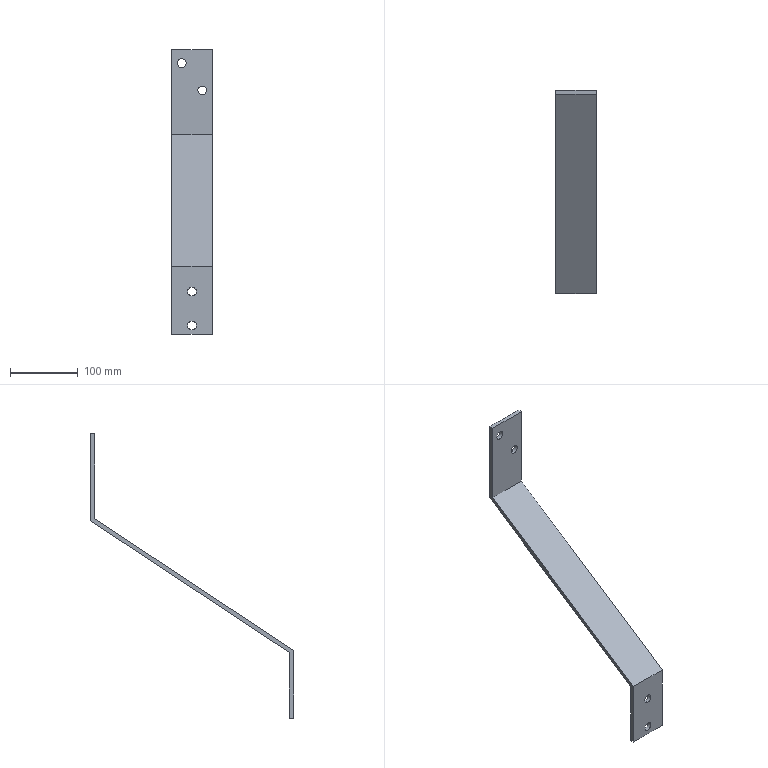Part | SolidWorks | features BaseBody 1 | 1 solid | 18 faces | box 60 x 299 x 419 mm | volume 204953 mm3 | plane 10 | cylinder 8 | commonest cylinder face diameters 13 x8
STEP:
#1=CARTESIAN_POINT('',(336.946,-3480.473,1530.471));
#2=VERTEX_POINT('',#1);
#3=CARTESIAN_POINT('',(336.946,-3480.473,1517.471));
#4=VERTEX_POINT('',#3);
#5=CARTESIAN_POINT('',(336.946,-3480.473,1523.971));
#6=DIRECTION('',(0.,-1.,0.));
#7=DIRECTION('',(0.,0.,-1.));
#8=AXIS2_PLACEMENT_3D('',#5,#6,#7);
#9=CIRCLE('',#8,6.5);
#10=EDGE_CURVE('',#2,#4,#9,.T.);
#11=ORIENTED_EDGE('',*,*,#10,.F.);
#12=CARTESIAN_POINT('',(336.946,-3486.473,1530.471));
#13=VERTEX_POINT('',#12);
#14=CARTESIAN_POINT('',(336.946,-3492.745,1530.471));
#15=DIRECTION('',(0.,-1.,0.));
#16=VECTOR('',#15,1000.);
#17=LINE('',#14,#16);
#18=EDGE_CURVE('',#2,#13,#17,.T.);
#19=ORIENTED_EDGE('',*,*,#18,.T.);
#20=CARTESIAN_POINT('',(336.946,-3486.473,1517.471));
#21=VERTEX_POINT('',#20);
#22=CARTESIAN_POINT('',(336.946,-3486.473,1523.971));
#23=DIRECTION('',(0.,1.,0.));
#24=DIRECTION('',(0.,0.,-1.));
#25=AXIS2_PLACEMENT_3D('',#22,#23,#24);
#26=CIRCLE('',#25,6.5);
#27=EDGE_CURVE('',#21,#13,#26,.T.);
#28=ORIENTED_EDGE('',*,*,#27,.F.);
#29=CARTESIAN_POINT('',(336.946,-3492.745,1517.471));
#30=DIRECTION('',(0.,-1.,0.));
#31=VECTOR('',#30,1000.);
#32=LINE('',#29,#31);
#33=EDGE_CURVE('',#4,#21,#32,.T.);
#34=ORIENTED_EDGE('',*,*,#33,.F.);
#35=EDGE_LOOP('',(#11,#19,#28,#34));
#36=FACE_OUTER_BOUND('',#35,.T.);
#37=CARTESIAN_POINT('',(336.946,-3492.745,1523.971));
#38=DIRECTION('',(0.,-1.,0.));
#39=DIRECTION('',(0.,0.,-1.));
#40=AXIS2_PLACEMENT_3D('',#37,#38,#39);
#41=CYLINDRICAL_SURFACE('',#40,6.5);
#42=ADVANCED_FACE('',(#36),#41,.F.);
#43=CARTESIAN_POINT('',(336.946,-3480.473,1580.471));
#44=VERTEX_POINT('',#43);
#45=CARTESIAN_POINT('',(336.946,-3480.473,1567.471));
#46=VERTEX_POINT('',#45);
#47=CARTESIAN_POINT('',(336.946,-3480.473,1573.971));
#48=DIRECTION('',(0.,-1.,0.));
#49=DIRECTION('',(0.,0.,-1.));
#50=AXIS2_PLACEMENT_3D('',#47,#48,#49);
#51=CIRCLE('',#50,6.5);
#52=EDGE_CURVE('',#44,#46,#51,.T.);
#53=ORIENTED_EDGE('',*,*,#52,.F.);
#54=CARTESIAN_POINT('',(336.946,-3486.473,1580.471));
#55=VERTEX_POINT('',#54);
#56=CARTESIAN_POINT('',(336.946,-3492.745,1580.471));
#57=DIRECTION('',(0.,-1.,0.));
#58=VECTOR('',#57,1000.);
#59=LINE('',#56,#58);
#60=EDGE_CURVE('',#44,#55,#59,.T.);
#61=ORIENTED_EDGE('',*,*,#60,.T.);
#62=CARTESIAN_POINT('',(336.946,-3486.473,1567.471));
#63=VERTEX_POINT('',#62);
#64=CARTESIAN_POINT('',(336.946,-3486.473,1573.971));
#65=DIRECTION('',(0.,1.,0.));
#66=DIRECTION('',(0.,0.,-1.));
#67=AXIS2_PLACEMENT_3D('',#64,#65,#66);
#68=CIRCLE('',#67,6.5);
#69=EDGE_CURVE('',#63,#55,#68,.T.);
#70=ORIENTED_EDGE('',*,*,#69,.F.);
#71=CARTESIAN_POINT('',(336.946,-3492.745,1567.471));
#72=DIRECTION('',(0.,-1.,0.));
#73=VECTOR('',#72,1000.);
#74=LINE('',#71,#73);
#75=EDGE_CURVE('',#46,#63,#74,.T.);
#76=ORIENTED_EDGE('',*,*,#75,.F.);
#77=EDGE_LOOP('',(#53,#61,#70,#76));
#78=FACE_OUTER_BOUND('',#77,.T.);
#79=CARTESIAN_POINT('',(336.946,-3492.745,1573.971));
#80=DIRECTION('',(0.,-1.,0.));
#81=DIRECTION('',(0.,0.,-1.));
#82=AXIS2_PLACEMENT_3D('',#79,#80,#81);
#83=CYLINDRICAL_SURFACE('',#82,6.5);
#84=ADVANCED_FACE('',(#78),#83,.F.);
#85=CARTESIAN_POINT('',(321.946,-3187.473,1916.471));
#86=VERTEX_POINT('',#85);
#87=CARTESIAN_POINT('',(321.946,-3187.473,1903.471));
#88=VERTEX_POINT('',#87);
#89=CARTESIAN_POINT('',(321.946,-3187.473,1909.971));
#90=DIRECTION('',(0.,-1.,0.));
#91=DIRECTION('',(0.,0.,-1.));
#92=AXIS2_PLACEMENT_3D('',#89,#90,#91);
#93=CIRCLE('',#92,6.5);
#94=EDGE_CURVE('',#86,#88,#93,.T.);
#95=ORIENTED_EDGE('',*,*,#94,.F.);
#96=CARTESIAN_POINT('',(321.946,-3193.473,1916.471));
#97=VERTEX_POINT('',#96);
#98=CARTESIAN_POINT('',(321.946,-3212.489,1916.471));
#99=DIRECTION('',(0.,-1.,0.));
#100=VECTOR('',#99,1000.);
#101=LINE('',#98,#100);
#102=EDGE_CURVE('',#86,#97,#101,.T.);
#103=ORIENTED_EDGE('',*,*,#102,.T.);
#104=CARTESIAN_POINT('',(321.946,-3193.473,1903.471));
#105=VERTEX_POINT('',#104);
#106=CARTESIAN_POINT('',(321.946,-3193.473,1909.971));
#107=DIRECTION('',(0.,1.,0.));
#108=DIRECTION('',(0.,0.,-1.));
#109=AXIS2_PLACEMENT_3D('',#106,#107,#108);
#110=CIRCLE('',#109,6.5);
#111=EDGE_CURVE('',#105,#97,#110,.T.);
#112=ORIENTED_EDGE('',*,*,#111,.F.);
#113=CARTESIAN_POINT('',(321.946,-3212.489,1903.471));
#114=DIRECTION('',(0.,-1.,0.));
#115=VECTOR('',#114,1000.);
#116=LINE('',#113,#115);
#117=EDGE_CURVE('',#88,#105,#116,.T.);
#118=ORIENTED_EDGE('',*,*,#117,.F.);
#119=EDGE_LOOP('',(#95,#103,#112,#118));
#120=FACE_OUTER_BOUND('',#119,.T.);
#121=CARTESIAN_POINT('',(321.946,-3212.489,1909.971));
#122=DIRECTION('',(0.,-1.,0.));
#123=DIRECTION('',(0.,0.,-1.));
#124=AXIS2_PLACEMENT_3D('',#121,#122,#123);
#125=CYLINDRICAL_SURFACE('',#124,6.5);
#126=ADVANCED_FACE('',(#120),#125,.F.);
#127=CARTESIAN_POINT('',(351.946,-3187.473,1876.471));
#128=VERTEX_POINT('',#127);
#129=CARTESIAN_POINT('',(351.946,-3187.473,1863.471));
#130=VERTEX_POINT('',#129);
#131=CARTESIAN_POINT('',(351.946,-3187.473,1869.971));
#132=DIRECTION('',(0.,-1.,0.));
#133=DIRECTION('',(0.,0.,-1.));
#134=AXIS2_PLACEMENT_3D('',#131,#132,#133);
#135=CIRCLE('',#134,6.5);
#136=EDGE_CURVE('',#128,#130,#135,.T.);
#137=ORIENTED_EDGE('',*,*,#136,.F.);
#138=CARTESIAN_POINT('',(351.946,-3193.473,1876.471));
#139=VERTEX_POINT('',#138);
#140=CARTESIAN_POINT('',(351.946,-3212.489,1876.471));
#141=DIRECTION('',(0.,-1.,0.));
#142=VECTOR('',#141,1000.);
#143=LINE('',#140,#142);
#144=EDGE_CURVE('',#128,#139,#143,.T.);
#145=ORIENTED_EDGE('',*,*,#144,.T.);
#146=CARTESIAN_POINT('',(351.946,-3193.473,1863.471));
#147=VERTEX_POINT('',#146);
#148=CARTESIAN_POINT('',(351.946,-3193.473,1869.971));
#149=DIRECTION('',(0.,1.,0.));
#150=DIRECTION('',(0.,0.,-1.));
#151=AXIS2_PLACEMENT_3D('',#148,#149,#150);
#152=CIRCLE('',#151,6.5);
#153=EDGE_CURVE('',#147,#139,#152,.T.);
#154=ORIENTED_EDGE('',*,*,#153,.F.);
#155=CARTESIAN_POINT('',(351.946,-3212.489,1863.471));
#156=DIRECTION('',(0.,-1.,0.));
#157=VECTOR('',#156,1000.);
#158=LINE('',#155,#157);
#159=EDGE_CURVE('',#130,#147,#158,.T.);
#160=ORIENTED_EDGE('',*,*,#159,.F.);
#161=EDGE_LOOP('',(#137,#145,#154,#160));
#162=FACE_OUTER_BOUND('',#161,.T.);
#163=CARTESIAN_POINT('',(351.946,-3212.489,1869.971));
#164=DIRECTION('',(0.,-1.,0.));
#165=DIRECTION('',(0.,0.,-1.));
#166=AXIS2_PLACEMENT_3D('',#163,#164,#165);
#167=CYLINDRICAL_SURFACE('',#166,6.5);
#168=ADVANCED_FACE('',(#162),#167,.F.);
#169=CARTESIAN_POINT('',(366.946,-3187.473,1801.712));
#170=VERTEX_POINT('',#169);
#171=CARTESIAN_POINT('',(366.946,-3480.473,1607.712));
#172=VERTEX_POINT('',#171);
#173=CARTESIAN_POINT('',(366.946,-3480.473,1607.712));
#174=DIRECTION('',(0.,-0.8338,-0.5521));
#175=VECTOR('',#174,1000.);
#176=LINE('',#173,#175);
#177=EDGE_CURVE('',#170,#172,#176,.T.);
#178=ORIENTED_EDGE('',*,*,#177,.T.);
#179=CARTESIAN_POINT('',(306.946,-3480.473,1607.712));
#180=VERTEX_POINT('',#179);
#181=CARTESIAN_POINT('',(366.946,-3480.473,1607.712));
#182=DIRECTION('',(-1.,0.,0.));
#183=VECTOR('',#182,1000.);
#184=LINE('',#181,#183);
#185=EDGE_CURVE('',#172,#180,#184,.T.);
#186=ORIENTED_EDGE('',*,*,#185,.T.);
#187=CARTESIAN_POINT('',(306.946,-3187.473,1801.712));
#188=VERTEX_POINT('',#187);
#189=CARTESIAN_POINT('',(306.946,-3480.473,1607.712));
#190=DIRECTION('',(0.,0.8338,0.5521));
#191=VECTOR('',#190,1000.);
#192=LINE('',#189,#191);
#193=EDGE_CURVE('',#180,#188,#192,.T.);
#194=ORIENTED_EDGE('',*,*,#193,.T.);
#195=CARTESIAN_POINT('',(366.946,-3187.473,1801.712));
#196=DIRECTION('',(1.,0.,0.));
#197=VECTOR('',#196,1000.);
#198=LINE('',#195,#197);
#199=EDGE_CURVE('',#188,#170,#198,.T.);
#200=ORIENTED_EDGE('',*,*,#199,.T.);
#201=EDGE_LOOP('',(#178,#186,#194,#200));
#202=FACE_OUTER_BOUND('',#201,.T.);
#203=CARTESIAN_POINT('',(366.946,-3480.473,1607.712));
#204=DIRECTION('',(0.,0.5521,-0.8338));
#205=DIRECTION('',(0.,0.8338,0.5521));
#206=AXIS2_PLACEMENT_3D('',#203,#204,#205);
#207=PLANE('',#206);
#208=ADVANCED_FACE('',(#202),#207,.T.);
#209=CARTESIAN_POINT('',(366.946,-3480.473,1510.971));
#210=VERTEX_POINT('',#209);
#211=CARTESIAN_POINT('',(366.946,-3480.473,1510.971));
#212=DIRECTION('',(0.,0.,-1.));
#213=VECTOR('',#212,1000.);
#214=LINE('',#211,#213);
#215=EDGE_CURVE('',#172,#210,#214,.T.);
#216=ORIENTED_EDGE('',*,*,#215,.T.);
#217=CARTESIAN_POINT('',(306.946,-3480.473,1510.971));
#218=VERTEX_POINT('',#217);
#219=CARTESIAN_POINT('',(366.946,-3480.473,1510.971));
#220=DIRECTION('',(-1.,0.,0.));
#221=VECTOR('',#220,1000.);
#222=LINE('',#219,#221);
#223=EDGE_CURVE('',#210,#218,#222,.T.);
#224=ORIENTED_EDGE('',*,*,#223,.T.);
#225=CARTESIAN_POINT('',(306.946,-3480.473,1510.971));
#226=DIRECTION('',(0.,0.,1.));
#227=VECTOR('',#226,1000.);
#228=LINE('',#225,#227);
#229=EDGE_CURVE('',#218,#180,#228,.T.);
#230=ORIENTED_EDGE('',*,*,#229,.T.);
#231=ORIENTED_EDGE('',*,*,#185,.F.);
#232=EDGE_LOOP('',(#216,#224,#230,#231));
#233=FACE_OUTER_BOUND('',#232,.T.);
#234=CARTESIAN_POINT('',(336.946,-3480.473,1523.971));
#235=DIRECTION('',(0.,-1.,0.));
#236=DIRECTION('',(0.,0.,-1.));
#237=AXIS2_PLACEMENT_3D('',#234,#235,#236);
#238=CIRCLE('',#237,6.5);
#239=EDGE_CURVE('',#4,#2,#238,.T.);
#240=ORIENTED_EDGE('',*,*,#239,.T.);
#241=ORIENTED_EDGE('',*,*,#10,.T.);
#242=EDGE_LOOP('',(#240,#241));
#243=FACE_BOUND('',#242,.T.);
#244=CARTESIAN_POINT('',(336.946,-3480.473,1573.971));
#245=DIRECTION('',(0.,-1.,0.));
#246=DIRECTION('',(0.,0.,-1.));
#247=AXIS2_PLACEMENT_3D('',#244,#245,#246);
#248=CIRCLE('',#247,6.5);
#249=EDGE_CURVE('',#46,#44,#248,.T.);
#250=ORIENTED_EDGE('',*,*,#249,.T.);
#251=ORIENTED_EDGE('',*,*,#52,.T.);
#252=EDGE_LOOP('',(#250,#251));
#253=FACE_BOUND('',#252,.T.);
#254=CARTESIAN_POINT('',(366.946,-3480.473,1510.971));
#255=DIRECTION('',(0.,1.,0.));
#256=DIRECTION('',(0.,0.,1.));
#257=AXIS2_PLACEMENT_3D('',#254,#255,#256);
#258=PLANE('',#257);
#259=ADVANCED_FACE('',(#233,#243,#253),#258,.T.);
#260=CARTESIAN_POINT('',(366.946,-3193.473,1804.971));
#261=VERTEX_POINT('',#260);
#262=CARTESIAN_POINT('',(366.946,-3486.473,1610.971));
#263=VERTEX_POINT('',#262);
#264=CARTESIAN_POINT('',(366.946,-3193.473,1804.971));
#265=DIRECTION('',(0.,-0.8338,-0.5521));
#266=VECTOR('',#265,1000.);
#267=LINE('',#264,#266);
#268=EDGE_CURVE('',#261,#263,#267,.T.);
#269=ORIENTED_EDGE('',*,*,#268,.T.);
#270=CARTESIAN_POINT('',(366.946,-3486.473,1510.971));
#271=VERTEX_POINT('',#270);
#272=CARTESIAN_POINT('',(366.946,-3486.473,1707.511));
#273=DIRECTION('',(0.,0.,-1.));
#274=VECTOR('',#273,1000.);
#275=LINE('',#272,#274);
#276=EDGE_CURVE('',#263,#271,#275,.T.);
#277=ORIENTED_EDGE('',*,*,#276,.T.);
#278=CARTESIAN_POINT('',(366.946,-3336.116,1510.971));
#279=DIRECTION('',(0.,1.,0.));
#280=VECTOR('',#279,1000.);
#281=LINE('',#278,#280);
#282=EDGE_CURVE('',#271,#210,#281,.T.);
#283=ORIENTED_EDGE('',*,*,#282,.T.);
#284=ORIENTED_EDGE('',*,*,#215,.F.);
#285=ORIENTED_EDGE('',*,*,#177,.F.);
#286=CARTESIAN_POINT('',(366.946,-3187.473,1929.971));
#287=VERTEX_POINT('',#286);
#288=CARTESIAN_POINT('',(366.946,-3187.473,1707.511));
#289=DIRECTION('',(0.,0.,1.));
#290=VECTOR('',#289,1000.);
#291=LINE('',#288,#290);
#292=EDGE_CURVE('',#170,#287,#291,.T.);
#293=ORIENTED_EDGE('',*,*,#292,.T.);
#294=CARTESIAN_POINT('',(366.946,-3193.473,1929.971));
#295=VERTEX_POINT('',#294);
#296=CARTESIAN_POINT('',(366.946,-3336.116,1929.971));
#297=DIRECTION('',(0.,-1.,0.));
#298=VECTOR('',#297,1000.);
#299=LINE('',#296,#298);
#300=EDGE_CURVE('',#287,#295,#299,.T.);
#301=ORIENTED_EDGE('',*,*,#300,.T.);
#302=CARTESIAN_POINT('',(366.946,-3193.473,1707.511));
#303=DIRECTION('',(0.,0.,-1.));
#304=VECTOR('',#303,1000.);
#305=LINE('',#302,#304);
#306=EDGE_CURVE('',#295,#261,#305,.T.);
#307=ORIENTED_EDGE('',*,*,#306,.T.);
#308=EDGE_LOOP('',(#269,#277,#283,#284,#285,#293,#301,#307));
#309=FACE_OUTER_BOUND('',#308,.T.);
#310=CARTESIAN_POINT('',(366.946,-3336.116,1707.511));
#311=DIRECTION('',(1.,0.,0.));
#312=DIRECTION('',(0.,1.,0.));
#313=AXIS2_PLACEMENT_3D('',#310,#311,#312);
#314=PLANE('',#313);
#315=ADVANCED_FACE('',(#309),#314,.T.);
#316=ORIENTED_EDGE('',*,*,#292,.F.);
#317=ORIENTED_EDGE('',*,*,#199,.F.);
#318=CARTESIAN_POINT('',(306.946,-3187.473,1929.971));
#319=VERTEX_POINT('',#318);
#320=CARTESIAN_POINT('',(306.946,-3187.473,1801.712));
#321=DIRECTION('',(0.,0.,1.));
#322=VECTOR('',#321,1000.);
#323=LINE('',#320,#322);
#324=EDGE_CURVE('',#188,#319,#323,.T.);
#325=ORIENTED_EDGE('',*,*,#324,.T.);
#326=CARTESIAN_POINT('',(366.946,-3187.473,1929.971));
#327=DIRECTION('',(1.,0.,0.));
#328=VECTOR('',#327,1000.);
#329=LINE('',#326,#328);
#330=EDGE_CURVE('',#319,#287,#329,.T.);
#331=ORIENTED_EDGE('',*,*,#330,.T.);
#332=EDGE_LOOP('',(#316,#317,#325,#331));
#333=FACE_OUTER_BOUND('',#332,.T.);
#334=CARTESIAN_POINT('',(321.946,-3187.473,1909.971));
#335=DIRECTION('',(0.,-1.,0.));
#336=DIRECTION('',(0.,0.,-1.));
#337=AXIS2_PLACEMENT_3D('',#334,#335,#336);
#338=CIRCLE('',#337,6.5);
#339=EDGE_CURVE('',#88,#86,#338,.T.);
#340=ORIENTED_EDGE('',*,*,#339,.T.);
#341=ORIENTED_EDGE('',*,*,#94,.T.);
#342=EDGE_LOOP('',(#340,#341));
#343=FACE_BOUND('',#342,.T.);
#344=CARTESIAN_POINT('',(351.946,-3187.473,1869.971));
#345=DIRECTION('',(0.,-1.,0.));
#346=DIRECTION('',(0.,0.,-1.));
#347=AXIS2_PLACEMENT_3D('',#344,#345,#346);
#348=CIRCLE('',#347,6.5);
#349=EDGE_CURVE('',#130,#128,#348,.T.);
#350=ORIENTED_EDGE('',*,*,#349,.T.);
#351=ORIENTED_EDGE('',*,*,#136,.T.);
#352=EDGE_LOOP('',(#350,#351));
#353=FACE_BOUND('',#352,.T.);
#354=CARTESIAN_POINT('',(366.946,-3187.473,1801.712));
#355=DIRECTION('',(0.,1.,0.));
#356=DIRECTION('',(0.,0.,1.));
#357=AXIS2_PLACEMENT_3D('',#354,#355,#356);
#358=PLANE('',#357);
#359=ADVANCED_FACE('',(#333,#343,#353),#358,.T.);
#360=CARTESIAN_POINT('',(306.946,-3486.473,1510.971));
#361=VERTEX_POINT('',#360);
#362=CARTESIAN_POINT('',(306.946,-3336.116,1510.971));
#363=DIRECTION('',(0.,1.,0.));
#364=VECTOR('',#363,1000.);
#365=LINE('',#362,#364);
#366=EDGE_CURVE('',#361,#218,#365,.T.);
#367=ORIENTED_EDGE('',*,*,#366,.F.);
#368=CARTESIAN_POINT('',(306.946,-3486.473,1610.971));
#369=VERTEX_POINT('',#368);
#370=CARTESIAN_POINT('',(306.946,-3486.473,1707.511));
#371=DIRECTION('',(0.,0.,-1.));
#372=VECTOR('',#371,1000.);
#373=LINE('',#370,#372);
#374=EDGE_CURVE('',#369,#361,#373,.T.);
#375=ORIENTED_EDGE('',*,*,#374,.F.);
#376=CARTESIAN_POINT('',(306.946,-3193.473,1804.971));
#377=VERTEX_POINT('',#376);
#378=CARTESIAN_POINT('',(306.946,-3193.473,1804.971));
#379=DIRECTION('',(0.,-0.8338,-0.5521));
#380=VECTOR('',#379,1000.);
#381=LINE('',#378,#380);
#382=EDGE_CURVE('',#377,#369,#381,.T.);
#383=ORIENTED_EDGE('',*,*,#382,.F.);
#384=CARTESIAN_POINT('',(306.946,-3193.473,1929.971));
#385=VERTEX_POINT('',#384);
#386=CARTESIAN_POINT('',(306.946,-3193.473,1707.511));
#387=DIRECTION('',(0.,0.,-1.));
#388=VECTOR('',#387,1000.);
#389=LINE('',#386,#388);
#390=EDGE_CURVE('',#385,#377,#389,.T.);
#391=ORIENTED_EDGE('',*,*,#390,.F.);
#392=CARTESIAN_POINT('',(306.946,-3336.116,1929.971));
#393=DIRECTION('',(0.,-1.,0.));
#394=VECTOR('',#393,1000.);
#395=LINE('',#392,#394);
#396=EDGE_CURVE('',#319,#385,#395,.T.);
#397=ORIENTED_EDGE('',*,*,#396,.F.);
#398=ORIENTED_EDGE('',*,*,#324,.F.);
#399=ORIENTED_EDGE('',*,*,#193,.F.);
#400=ORIENTED_EDGE('',*,*,#229,.F.);
#401=EDGE_LOOP('',(#367,#375,#383,#391,#397,#398,#399,#400));
#402=FACE_OUTER_BOUND('',#401,.T.);
#403=CARTESIAN_POINT('',(306.946,-3336.116,1707.511));
#404=DIRECTION('',(1.,0.,0.));
#405=DIRECTION('',(0.,1.,0.));
#406=AXIS2_PLACEMENT_3D('',#403,#404,#405);
#407=PLANE('',#406);
#408=ADVANCED_FACE('',(#402),#407,.F.);
#409=ORIENTED_EDGE('',*,*,#282,.F.);
#410=CARTESIAN_POINT('',(366.946,-3486.473,1510.971));
#411=DIRECTION('',(-1.,0.,0.));
#412=VECTOR('',#411,1000.);
#413=LINE('',#410,#412);
#414=EDGE_CURVE('',#271,#361,#413,.T.);
#415=ORIENTED_EDGE('',*,*,#414,.T.);
#416=ORIENTED_EDGE('',*,*,#366,.T.);
#417=ORIENTED_EDGE('',*,*,#223,.F.);
#418=EDGE_LOOP('',(#409,#415,#416,#417));
#419=FACE_OUTER_BOUND('',#418,.T.);
#420=CARTESIAN_POINT('',(366.946,-3486.473,1510.971));
#421=DIRECTION('',(0.,0.,-1.));
#422=DIRECTION('',(-1.,0.,0.));
#423=AXIS2_PLACEMENT_3D('',#420,#421,#422);
#424=PLANE('',#423);
#425=ADVANCED_FACE('',(#419),#424,.T.);
#426=ORIENTED_EDGE('',*,*,#18,.F.);
#427=ORIENTED_EDGE('',*,*,#239,.F.);
#428=ORIENTED_EDGE('',*,*,#33,.T.);
#429=CARTESIAN_POINT('',(336.946,-3486.473,1523.971));
#430=DIRECTION('',(0.,1.,0.));
#431=DIRECTION('',(0.,0.,-1.));
#432=AXIS2_PLACEMENT_3D('',#429,#430,#431);
#433=CIRCLE('',#432,6.5);
#434=EDGE_CURVE('',#13,#21,#433,.T.);
#435=ORIENTED_EDGE('',*,*,#434,.F.);
#436=EDGE_LOOP('',(#426,#427,#428,#435));
#437=FACE_OUTER_BOUND('',#436,.T.);
#438=CARTESIAN_POINT('',(336.946,-3492.745,1523.971));
#439=DIRECTION('',(0.,-1.,0.));
#440=DIRECTION('',(0.,0.,-1.));
#441=AXIS2_PLACEMENT_3D('',#438,#439,#440);
#442=CYLINDRICAL_SURFACE('',#441,6.5);
#443=ADVANCED_FACE('',(#437),#442,.F.);
#444=ORIENTED_EDGE('',*,*,#60,.F.);
#445=ORIENTED_EDGE('',*,*,#249,.F.);
#446=ORIENTED_EDGE('',*,*,#75,.T.);
#447=CARTESIAN_POINT('',(336.946,-3486.473,1573.971));
#448=DIRECTION('',(0.,1.,0.));
#449=DIRECTION('',(0.,0.,-1.));
#450=AXIS2_PLACEMENT_3D('',#447,#448,#449);
#451=CIRCLE('',#450,6.5);
#452=EDGE_CURVE('',#55,#63,#451,.T.);
#453=ORIENTED_EDGE('',*,*,#452,.F.);
#454=EDGE_LOOP('',(#444,#445,#446,#453));
#455=FACE_OUTER_BOUND('',#454,.T.);
#456=CARTESIAN_POINT('',(336.946,-3492.745,1573.971));
#457=DIRECTION('',(0.,-1.,0.));
#458=DIRECTION('',(0.,0.,-1.));
#459=AXIS2_PLACEMENT_3D('',#456,#457,#458);
#460=CYLINDRICAL_SURFACE('',#459,6.5);
#461=ADVANCED_FACE('',(#455),#460,.F.);
#462=ORIENTED_EDGE('',*,*,#276,.F.);
#463=CARTESIAN_POINT('',(366.946,-3486.473,1610.971));
#464=DIRECTION('',(-1.,0.,0.));
#465=VECTOR('',#464,1000.);
#466=LINE('',#463,#465);
#467=EDGE_CURVE('',#263,#369,#466,.T.);
#468=ORIENTED_EDGE('',*,*,#467,.T.);
#469=ORIENTED_EDGE('',*,*,#374,.T.);
#470=ORIENTED_EDGE('',*,*,#414,.F.);
#471=EDGE_LOOP('',(#462,#468,#469,#470));
#472=FACE_OUTER_BOUND('',#471,.T.);
#473=ORIENTED_EDGE('',*,*,#27,.T.);
#474=ORIENTED_EDGE('',*,*,#434,.T.);
#475=EDGE_LOOP('',(#473,#474));
#476=FACE_BOUND('',#475,.T.);
#477=ORIENTED_EDGE('',*,*,#69,.T.);
#478=ORIENTED_EDGE('',*,*,#452,.T.);
#479=EDGE_LOOP('',(#477,#478));
#480=FACE_BOUND('',#479,.T.);
#481=CARTESIAN_POINT('',(366.946,-3486.473,1610.971));
#482=DIRECTION('',(0.,-1.,0.));
#483=DIRECTION('',(0.,0.,-1.));
#484=AXIS2_PLACEMENT_3D('',#481,#482,#483);
#485=PLANE('',#484);
#486=ADVANCED_FACE('',(#472,#476,#480),#485,.T.);
#487=ORIENTED_EDGE('',*,*,#268,.F.);
#488=CARTESIAN_POINT('',(366.946,-3193.473,1804.971));
#489=DIRECTION('',(-1.,0.,0.));
#490=VECTOR('',#489,1000.);
#491=LINE('',#488,#490);
#492=EDGE_CURVE('',#261,#377,#491,.T.);
#493=ORIENTED_EDGE('',*,*,#492,.T.);
#494=ORIENTED_EDGE('',*,*,#382,.T.);
#495=ORIENTED_EDGE('',*,*,#467,.F.);
#496=EDGE_LOOP('',(#487,#493,#494,#495));
#497=FACE_OUTER_BOUND('',#496,.T.);
#498=CARTESIAN_POINT('',(366.946,-3193.473,1804.971));
#499=DIRECTION('',(0.,-0.5521,0.8338));
#500=DIRECTION('',(0.,-0.8338,-0.5521));
#501=AXIS2_PLACEMENT_3D('',#498,#499,#500);
#502=PLANE('',#501);
#503=ADVANCED_FACE('',(#497),#502,.T.);
#504=ORIENTED_EDGE('',*,*,#306,.F.);
#505=CARTESIAN_POINT('',(366.946,-3193.473,1929.971));
#506=DIRECTION('',(-1.,0.,0.));
#507=VECTOR('',#506,1000.);
#508=LINE('',#505,#507);
#509=EDGE_CURVE('',#295,#385,#508,.T.);
#510=ORIENTED_EDGE('',*,*,#509,.T.);
#511=ORIENTED_EDGE('',*,*,#390,.T.);
#512=ORIENTED_EDGE('',*,*,#492,.F.);
#513=EDGE_LOOP('',(#504,#510,#511,#512));
#514=FACE_OUTER_BOUND('',#513,.T.);
#515=ORIENTED_EDGE('',*,*,#111,.T.);
#516=CARTESIAN_POINT('',(321.946,-3193.473,1909.971));
#517=DIRECTION('',(0.,1.,0.));
#518=DIRECTION('',(0.,0.,-1.));
#519=AXIS2_PLACEMENT_3D('',#516,#517,#518);
#520=CIRCLE('',#519,6.5);
#521=EDGE_CURVE('',#97,#105,#520,.T.);
#522=ORIENTED_EDGE('',*,*,#521,.T.);
#523=EDGE_LOOP('',(#515,#522));
#524=FACE_BOUND('',#523,.T.);
#525=ORIENTED_EDGE('',*,*,#153,.T.);
#526=CARTESIAN_POINT('',(351.946,-3193.473,1869.971));
#527=DIRECTION('',(0.,1.,0.));
#528=DIRECTION('',(0.,0.,-1.));
#529=AXIS2_PLACEMENT_3D('',#526,#527,#528);
#530=CIRCLE('',#529,6.5);
#531=EDGE_CURVE('',#139,#147,#530,.T.);
#532=ORIENTED_EDGE('',*,*,#531,.T.);
#533=EDGE_LOOP('',(#525,#532));
#534=FACE_BOUND('',#533,.T.);
#535=CARTESIAN_POINT('',(366.946,-3193.473,1904.971));
#536=DIRECTION('',(0.,-1.,0.));
#537=DIRECTION('',(0.,0.,-1.));
#538=AXIS2_PLACEMENT_3D('',#535,#536,#537);
#539=PLANE('',#538);
#540=ADVANCED_FACE('',(#514,#524,#534),#539,.T.);
#541=ORIENTED_EDGE('',*,*,#300,.F.);
#542=ORIENTED_EDGE('',*,*,#330,.F.);
#543=ORIENTED_EDGE('',*,*,#396,.T.);
#544=ORIENTED_EDGE('',*,*,#509,.F.);
#545=EDGE_LOOP('',(#541,#542,#543,#544));
#546=FACE_OUTER_BOUND('',#545,.T.);
#547=CARTESIAN_POINT('',(366.946,-3187.473,1929.971));
#548=DIRECTION('',(0.,0.,1.));
#549=DIRECTION('',(1.,0.,0.));
#550=AXIS2_PLACEMENT_3D('',#547,#548,#549);
#551=PLANE('',#550);
#552=ADVANCED_FACE('',(#546),#551,.T.);
#553=ORIENTED_EDGE('',*,*,#102,.F.);
#554=ORIENTED_EDGE('',*,*,#339,.F.);
#555=ORIENTED_EDGE('',*,*,#117,.T.);
#556=ORIENTED_EDGE('',*,*,#521,.F.);
#557=EDGE_LOOP('',(#553,#554,#555,#556));
#558=FACE_OUTER_BOUND('',#557,.T.);
#559=CARTESIAN_POINT('',(321.946,-3212.489,1909.971));
#560=DIRECTION('',(0.,-1.,0.));
#561=DIRECTION('',(0.,0.,-1.));
#562=AXIS2_PLACEMENT_3D('',#559,#560,#561);
#563=CYLINDRICAL_SURFACE('',#562,6.5);
#564=ADVANCED_FACE('',(#558),#563,.F.);
#565=ORIENTED_EDGE('',*,*,#144,.F.);
#566=ORIENTED_EDGE('',*,*,#349,.F.);
#567=ORIENTED_EDGE('',*,*,#159,.T.);
#568=ORIENTED_EDGE('',*,*,#531,.F.);
#569=EDGE_LOOP('',(#565,#566,#567,#568));
#570=FACE_OUTER_BOUND('',#569,.T.);
#571=CARTESIAN_POINT('',(351.946,-3212.489,1869.971));
#572=DIRECTION('',(0.,-1.,0.));
#573=DIRECTION('',(0.,0.,-1.));
#574=AXIS2_PLACEMENT_3D('',#571,#572,#573);
#575=CYLINDRICAL_SURFACE('',#574,6.5);
#576=ADVANCED_FACE('',(#570),#575,.F.);
#577=CLOSED_SHELL('',(#42,#84,#126,#168,#208,#259,#315,#359,#408,#425,#443,#461,#486,#503,#540,#552,#564,#576));
#578=MANIFOLD_SOLID_BREP('',#577);
#579=CARTESIAN_POINT('',(0.,0.,0.));
#580=DIRECTION('',(0.,0.,1.));
#581=DIRECTION('',(1.,0.,0.));
#582=AXIS2_PLACEMENT_3D('',#579,#580,#581);
#583=(LENGTH_UNIT()NAMED_UNIT(*)SI_UNIT(.MILLI.,.METRE.));
#584=UNCERTAINTY_MEASURE_WITH_UNIT(LENGTH_MEASURE(0.00001),#583,'','');
#585=(NAMED_UNIT(*)PLANE_ANGLE_UNIT()SI_UNIT($,.RADIAN.));
#586=(NAMED_UNIT(*)SI_UNIT($,.STERADIAN.)SOLID_ANGLE_UNIT());
#587=(GEOMETRIC_REPRESENTATION_CONTEXT(3)GLOBAL_UNCERTAINTY_ASSIGNED_CONTEXT((#584))GLOBAL_UNIT_ASSIGNED_CONTEXT((#583,#585,#586))REPRESENTATION_CONTEXT('',''));
#588=ADVANCED_BREP_SHAPE_REPRESENTATION('',(#578,#582),#587);